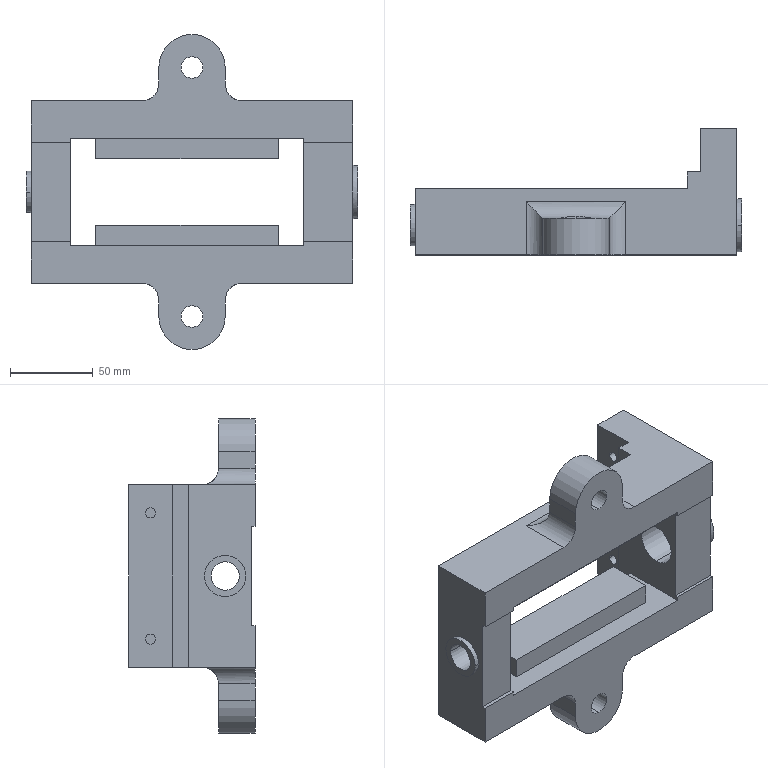Part | SolidWorks | features ICE 10, Extrusion 1, Fillet 1, MirrorSolid 1 | 1 solid | 68 faces | box 200 x 76 x 190 mm | volume 696258 mm3 | plane 40 | cylinder 28 | commonest cylinder face diameters 20 x6 6 x4 13 x4 25 x4 30 x4 17 x2